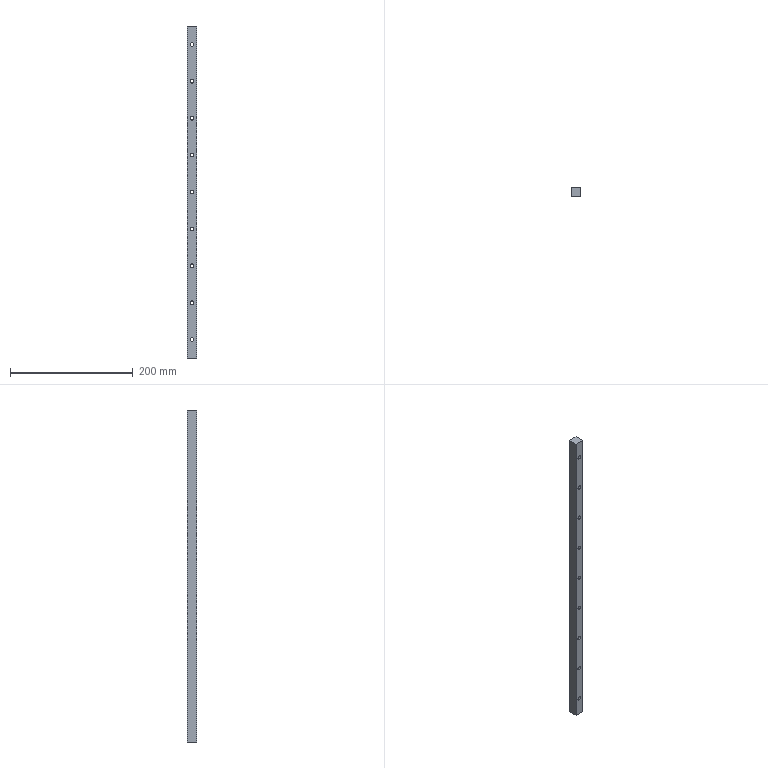Part | 1 solid | 24 faces | box 15 x 15 x 540 mm | volume 117683 mm3 | cylinder 18 | plane 6 | commonest cylinder face diameters 6 x18
STEP:
#1=CARTESIAN_POINT('',(7.5,0.,507.));
#2=VERTEX_POINT('',#1);
#3=CARTESIAN_POINT('',(7.5,0.,513.));
#4=VERTEX_POINT('',#3);
#5=CARTESIAN_POINT('',(7.5,0.,510.));
#6=DIRECTION('',(0.,1.,0.));
#7=DIRECTION('',(0.,0.,1.));
#8=AXIS2_PLACEMENT_3D('',#5,#6,#7);
#9=CIRCLE('',#8,3.);
#10=EDGE_CURVE('',#2,#4,#9,.T.);
#11=ORIENTED_EDGE('',*,*,#10,.F.);
#12=CARTESIAN_POINT('',(7.5,15.,507.));
#13=VERTEX_POINT('',#12);
#14=CARTESIAN_POINT('',(7.5,-35.,507.));
#15=DIRECTION('',(0.,1.,0.));
#16=VECTOR('',#15,1000.);
#17=LINE('',#14,#16);
#18=EDGE_CURVE('',#2,#13,#17,.T.);
#19=ORIENTED_EDGE('',*,*,#18,.T.);
#20=CARTESIAN_POINT('',(7.5,15.,513.));
#21=VERTEX_POINT('',#20);
#22=CARTESIAN_POINT('',(7.5,15.,510.));
#23=DIRECTION('',(0.,1.,0.));
#24=DIRECTION('',(0.,0.,1.));
#25=AXIS2_PLACEMENT_3D('',#22,#23,#24);
#26=CIRCLE('',#25,3.);
#27=EDGE_CURVE('',#13,#21,#26,.T.);
#28=ORIENTED_EDGE('',*,*,#27,.T.);
#29=CARTESIAN_POINT('',(7.5,-35.,513.));
#30=DIRECTION('',(0.,1.,0.));
#31=VECTOR('',#30,1000.);
#32=LINE('',#29,#31);
#33=EDGE_CURVE('',#4,#21,#32,.T.);
#34=ORIENTED_EDGE('',*,*,#33,.F.);
#35=EDGE_LOOP('',(#11,#19,#28,#34));
#36=FACE_OUTER_BOUND('',#35,.T.);
#37=CARTESIAN_POINT('',(7.5,-35.,510.));
#38=DIRECTION('',(0.,1.,0.));
#39=DIRECTION('',(0.,0.,1.));
#40=AXIS2_PLACEMENT_3D('',#37,#38,#39);
#41=CYLINDRICAL_SURFACE('',#40,3.);
#42=ADVANCED_FACE('',(#36),#41,.F.);
#43=CARTESIAN_POINT('',(7.5,0.,447.));
#44=VERTEX_POINT('',#43);
#45=CARTESIAN_POINT('',(7.5,0.,453.));
#46=VERTEX_POINT('',#45);
#47=CARTESIAN_POINT('',(7.5,0.,450.));
#48=DIRECTION('',(0.,1.,0.));
#49=DIRECTION('',(0.,0.,1.));
#50=AXIS2_PLACEMENT_3D('',#47,#48,#49);
#51=CIRCLE('',#50,3.);
#52=EDGE_CURVE('',#44,#46,#51,.T.);
#53=ORIENTED_EDGE('',*,*,#52,.F.);
#54=CARTESIAN_POINT('',(7.5,15.,447.));
#55=VERTEX_POINT('',#54);
#56=CARTESIAN_POINT('',(7.5,-35.,447.));
#57=DIRECTION('',(0.,1.,0.));
#58=VECTOR('',#57,1000.);
#59=LINE('',#56,#58);
#60=EDGE_CURVE('',#44,#55,#59,.T.);
#61=ORIENTED_EDGE('',*,*,#60,.T.);
#62=CARTESIAN_POINT('',(7.5,15.,453.));
#63=VERTEX_POINT('',#62);
#64=CARTESIAN_POINT('',(7.5,15.,450.));
#65=DIRECTION('',(0.,1.,0.));
#66=DIRECTION('',(0.,0.,1.));
#67=AXIS2_PLACEMENT_3D('',#64,#65,#66);
#68=CIRCLE('',#67,3.);
#69=EDGE_CURVE('',#55,#63,#68,.T.);
#70=ORIENTED_EDGE('',*,*,#69,.T.);
#71=CARTESIAN_POINT('',(7.5,-35.,453.));
#72=DIRECTION('',(0.,1.,0.));
#73=VECTOR('',#72,1000.);
#74=LINE('',#71,#73);
#75=EDGE_CURVE('',#46,#63,#74,.T.);
#76=ORIENTED_EDGE('',*,*,#75,.F.);
#77=EDGE_LOOP('',(#53,#61,#70,#76));
#78=FACE_OUTER_BOUND('',#77,.T.);
#79=CARTESIAN_POINT('',(7.5,-35.,450.));
#80=DIRECTION('',(0.,1.,0.));
#81=DIRECTION('',(0.,0.,1.));
#82=AXIS2_PLACEMENT_3D('',#79,#80,#81);
#83=CYLINDRICAL_SURFACE('',#82,3.);
#84=ADVANCED_FACE('',(#78),#83,.F.);
#85=CARTESIAN_POINT('',(7.5,0.,387.));
#86=VERTEX_POINT('',#85);
#87=CARTESIAN_POINT('',(7.5,0.,393.));
#88=VERTEX_POINT('',#87);
#89=CARTESIAN_POINT('',(7.5,0.,390.));
#90=DIRECTION('',(0.,1.,0.));
#91=DIRECTION('',(0.,0.,1.));
#92=AXIS2_PLACEMENT_3D('',#89,#90,#91);
#93=CIRCLE('',#92,3.);
#94=EDGE_CURVE('',#86,#88,#93,.T.);
#95=ORIENTED_EDGE('',*,*,#94,.F.);
#96=CARTESIAN_POINT('',(7.5,15.,387.));
#97=VERTEX_POINT('',#96);
#98=CARTESIAN_POINT('',(7.5,-35.,387.));
#99=DIRECTION('',(0.,1.,0.));
#100=VECTOR('',#99,1000.);
#101=LINE('',#98,#100);
#102=EDGE_CURVE('',#86,#97,#101,.T.);
#103=ORIENTED_EDGE('',*,*,#102,.T.);
#104=CARTESIAN_POINT('',(7.5,15.,393.));
#105=VERTEX_POINT('',#104);
#106=CARTESIAN_POINT('',(7.5,15.,390.));
#107=DIRECTION('',(0.,1.,0.));
#108=DIRECTION('',(0.,0.,1.));
#109=AXIS2_PLACEMENT_3D('',#106,#107,#108);
#110=CIRCLE('',#109,3.);
#111=EDGE_CURVE('',#97,#105,#110,.T.);
#112=ORIENTED_EDGE('',*,*,#111,.T.);
#113=CARTESIAN_POINT('',(7.5,-35.,393.));
#114=DIRECTION('',(0.,1.,0.));
#115=VECTOR('',#114,1000.);
#116=LINE('',#113,#115);
#117=EDGE_CURVE('',#88,#105,#116,.T.);
#118=ORIENTED_EDGE('',*,*,#117,.F.);
#119=EDGE_LOOP('',(#95,#103,#112,#118));
#120=FACE_OUTER_BOUND('',#119,.T.);
#121=CARTESIAN_POINT('',(7.5,-35.,390.));
#122=DIRECTION('',(0.,1.,0.));
#123=DIRECTION('',(0.,0.,1.));
#124=AXIS2_PLACEMENT_3D('',#121,#122,#123);
#125=CYLINDRICAL_SURFACE('',#124,3.);
#126=ADVANCED_FACE('',(#120),#125,.F.);
#127=CARTESIAN_POINT('',(7.5,0.,327.));
#128=VERTEX_POINT('',#127);
#129=CARTESIAN_POINT('',(7.5,0.,333.));
#130=VERTEX_POINT('',#129);
#131=CARTESIAN_POINT('',(7.5,0.,330.));
#132=DIRECTION('',(0.,1.,0.));
#133=DIRECTION('',(0.,0.,1.));
#134=AXIS2_PLACEMENT_3D('',#131,#132,#133);
#135=CIRCLE('',#134,3.);
#136=EDGE_CURVE('',#128,#130,#135,.T.);
#137=ORIENTED_EDGE('',*,*,#136,.F.);
#138=CARTESIAN_POINT('',(7.5,15.,327.));
#139=VERTEX_POINT('',#138);
#140=CARTESIAN_POINT('',(7.5,-35.,327.));
#141=DIRECTION('',(0.,1.,0.));
#142=VECTOR('',#141,1000.);
#143=LINE('',#140,#142);
#144=EDGE_CURVE('',#128,#139,#143,.T.);
#145=ORIENTED_EDGE('',*,*,#144,.T.);
#146=CARTESIAN_POINT('',(7.5,15.,333.));
#147=VERTEX_POINT('',#146);
#148=CARTESIAN_POINT('',(7.5,15.,330.));
#149=DIRECTION('',(0.,1.,0.));
#150=DIRECTION('',(0.,0.,1.));
#151=AXIS2_PLACEMENT_3D('',#148,#149,#150);
#152=CIRCLE('',#151,3.);
#153=EDGE_CURVE('',#139,#147,#152,.T.);
#154=ORIENTED_EDGE('',*,*,#153,.T.);
#155=CARTESIAN_POINT('',(7.5,-35.,333.));
#156=DIRECTION('',(0.,1.,0.));
#157=VECTOR('',#156,1000.);
#158=LINE('',#155,#157);
#159=EDGE_CURVE('',#130,#147,#158,.T.);
#160=ORIENTED_EDGE('',*,*,#159,.F.);
#161=EDGE_LOOP('',(#137,#145,#154,#160));
#162=FACE_OUTER_BOUND('',#161,.T.);
#163=CARTESIAN_POINT('',(7.5,-35.,330.));
#164=DIRECTION('',(0.,1.,0.));
#165=DIRECTION('',(0.,0.,1.));
#166=AXIS2_PLACEMENT_3D('',#163,#164,#165);
#167=CYLINDRICAL_SURFACE('',#166,3.);
#168=ADVANCED_FACE('',(#162),#167,.F.);
#169=CARTESIAN_POINT('',(7.5,0.,267.));
#170=VERTEX_POINT('',#169);
#171=CARTESIAN_POINT('',(7.5,0.,273.));
#172=VERTEX_POINT('',#171);
#173=CARTESIAN_POINT('',(7.5,0.,270.));
#174=DIRECTION('',(0.,1.,0.));
#175=DIRECTION('',(0.,0.,1.));
#176=AXIS2_PLACEMENT_3D('',#173,#174,#175);
#177=CIRCLE('',#176,3.);
#178=EDGE_CURVE('',#170,#172,#177,.T.);
#179=ORIENTED_EDGE('',*,*,#178,.F.);
#180=CARTESIAN_POINT('',(7.5,15.,267.));
#181=VERTEX_POINT('',#180);
#182=CARTESIAN_POINT('',(7.5,-35.,267.));
#183=DIRECTION('',(0.,1.,0.));
#184=VECTOR('',#183,1000.);
#185=LINE('',#182,#184);
#186=EDGE_CURVE('',#170,#181,#185,.T.);
#187=ORIENTED_EDGE('',*,*,#186,.T.);
#188=CARTESIAN_POINT('',(7.5,15.,273.));
#189=VERTEX_POINT('',#188);
#190=CARTESIAN_POINT('',(7.5,15.,270.));
#191=DIRECTION('',(0.,1.,0.));
#192=DIRECTION('',(0.,0.,1.));
#193=AXIS2_PLACEMENT_3D('',#190,#191,#192);
#194=CIRCLE('',#193,3.);
#195=EDGE_CURVE('',#181,#189,#194,.T.);
#196=ORIENTED_EDGE('',*,*,#195,.T.);
#197=CARTESIAN_POINT('',(7.5,-35.,273.));
#198=DIRECTION('',(0.,1.,0.));
#199=VECTOR('',#198,1000.);
#200=LINE('',#197,#199);
#201=EDGE_CURVE('',#172,#189,#200,.T.);
#202=ORIENTED_EDGE('',*,*,#201,.F.);
#203=EDGE_LOOP('',(#179,#187,#196,#202));
#204=FACE_OUTER_BOUND('',#203,.T.);
#205=CARTESIAN_POINT('',(7.5,-35.,270.));
#206=DIRECTION('',(0.,1.,0.));
#207=DIRECTION('',(0.,0.,1.));
#208=AXIS2_PLACEMENT_3D('',#205,#206,#207);
#209=CYLINDRICAL_SURFACE('',#208,3.);
#210=ADVANCED_FACE('',(#204),#209,.F.);
#211=CARTESIAN_POINT('',(7.5,0.,207.));
#212=VERTEX_POINT('',#211);
#213=CARTESIAN_POINT('',(7.5,0.,213.));
#214=VERTEX_POINT('',#213);
#215=CARTESIAN_POINT('',(7.5,0.,210.));
#216=DIRECTION('',(0.,1.,0.));
#217=DIRECTION('',(0.,0.,1.));
#218=AXIS2_PLACEMENT_3D('',#215,#216,#217);
#219=CIRCLE('',#218,3.);
#220=EDGE_CURVE('',#212,#214,#219,.T.);
#221=ORIENTED_EDGE('',*,*,#220,.F.);
#222=CARTESIAN_POINT('',(7.5,15.,207.));
#223=VERTEX_POINT('',#222);
#224=CARTESIAN_POINT('',(7.5,-35.,207.));
#225=DIRECTION('',(0.,1.,0.));
#226=VECTOR('',#225,1000.);
#227=LINE('',#224,#226);
#228=EDGE_CURVE('',#212,#223,#227,.T.);
#229=ORIENTED_EDGE('',*,*,#228,.T.);
#230=CARTESIAN_POINT('',(7.5,15.,213.));
#231=VERTEX_POINT('',#230);
#232=CARTESIAN_POINT('',(7.5,15.,210.));
#233=DIRECTION('',(0.,1.,0.));
#234=DIRECTION('',(0.,0.,1.));
#235=AXIS2_PLACEMENT_3D('',#232,#233,#234);
#236=CIRCLE('',#235,3.);
#237=EDGE_CURVE('',#223,#231,#236,.T.);
#238=ORIENTED_EDGE('',*,*,#237,.T.);
#239=CARTESIAN_POINT('',(7.5,-35.,213.));
#240=DIRECTION('',(0.,1.,0.));
#241=VECTOR('',#240,1000.);
#242=LINE('',#239,#241);
#243=EDGE_CURVE('',#214,#231,#242,.T.);
#244=ORIENTED_EDGE('',*,*,#243,.F.);
#245=EDGE_LOOP('',(#221,#229,#238,#244));
#246=FACE_OUTER_BOUND('',#245,.T.);
#247=CARTESIAN_POINT('',(7.5,-35.,210.));
#248=DIRECTION('',(0.,1.,0.));
#249=DIRECTION('',(0.,0.,1.));
#250=AXIS2_PLACEMENT_3D('',#247,#248,#249);
#251=CYLINDRICAL_SURFACE('',#250,3.);
#252=ADVANCED_FACE('',(#246),#251,.F.);
#253=CARTESIAN_POINT('',(7.5,0.,147.));
#254=VERTEX_POINT('',#253);
#255=CARTESIAN_POINT('',(7.5,0.,153.));
#256=VERTEX_POINT('',#255);
#257=CARTESIAN_POINT('',(7.5,0.,150.));
#258=DIRECTION('',(0.,1.,0.));
#259=DIRECTION('',(0.,0.,1.));
#260=AXIS2_PLACEMENT_3D('',#257,#258,#259);
#261=CIRCLE('',#260,3.);
#262=EDGE_CURVE('',#254,#256,#261,.T.);
#263=ORIENTED_EDGE('',*,*,#262,.F.);
#264=CARTESIAN_POINT('',(7.5,15.,147.));
#265=VERTEX_POINT('',#264);
#266=CARTESIAN_POINT('',(7.5,-35.,147.));
#267=DIRECTION('',(0.,1.,0.));
#268=VECTOR('',#267,1000.);
#269=LINE('',#266,#268);
#270=EDGE_CURVE('',#254,#265,#269,.T.);
#271=ORIENTED_EDGE('',*,*,#270,.T.);
#272=CARTESIAN_POINT('',(7.5,15.,153.));
#273=VERTEX_POINT('',#272);
#274=CARTESIAN_POINT('',(7.5,15.,150.));
#275=DIRECTION('',(0.,1.,0.));
#276=DIRECTION('',(0.,0.,1.));
#277=AXIS2_PLACEMENT_3D('',#274,#275,#276);
#278=CIRCLE('',#277,3.);
#279=EDGE_CURVE('',#265,#273,#278,.T.);
#280=ORIENTED_EDGE('',*,*,#279,.T.);
#281=CARTESIAN_POINT('',(7.5,-35.,153.));
#282=DIRECTION('',(0.,1.,0.));
#283=VECTOR('',#282,1000.);
#284=LINE('',#281,#283);
#285=EDGE_CURVE('',#256,#273,#284,.T.);
#286=ORIENTED_EDGE('',*,*,#285,.F.);
#287=EDGE_LOOP('',(#263,#271,#280,#286));
#288=FACE_OUTER_BOUND('',#287,.T.);
#289=CARTESIAN_POINT('',(7.5,-35.,150.));
#290=DIRECTION('',(0.,1.,0.));
#291=DIRECTION('',(0.,0.,1.));
#292=AXIS2_PLACEMENT_3D('',#289,#290,#291);
#293=CYLINDRICAL_SURFACE('',#292,3.);
#294=ADVANCED_FACE('',(#288),#293,.F.);
#295=CARTESIAN_POINT('',(7.5,0.,87.));
#296=VERTEX_POINT('',#295);
#297=CARTESIAN_POINT('',(7.5,0.,93.));
#298=VERTEX_POINT('',#297);
#299=CARTESIAN_POINT('',(7.5,0.,90.));
#300=DIRECTION('',(0.,1.,0.));
#301=DIRECTION('',(0.,0.,1.));
#302=AXIS2_PLACEMENT_3D('',#299,#300,#301);
#303=CIRCLE('',#302,3.);
#304=EDGE_CURVE('',#296,#298,#303,.T.);
#305=ORIENTED_EDGE('',*,*,#304,.F.);
#306=CARTESIAN_POINT('',(7.5,15.,87.));
#307=VERTEX_POINT('',#306);
#308=CARTESIAN_POINT('',(7.5,-35.,87.));
#309=DIRECTION('',(0.,1.,0.));
#310=VECTOR('',#309,1000.);
#311=LINE('',#308,#310);
#312=EDGE_CURVE('',#296,#307,#311,.T.);
#313=ORIENTED_EDGE('',*,*,#312,.T.);
#314=CARTESIAN_POINT('',(7.5,15.,93.));
#315=VERTEX_POINT('',#314);
#316=CARTESIAN_POINT('',(7.5,15.,90.));
#317=DIRECTION('',(0.,1.,0.));
#318=DIRECTION('',(0.,0.,1.));
#319=AXIS2_PLACEMENT_3D('',#316,#317,#318);
#320=CIRCLE('',#319,3.);
#321=EDGE_CURVE('',#307,#315,#320,.T.);
#322=ORIENTED_EDGE('',*,*,#321,.T.);
#323=CARTESIAN_POINT('',(7.5,-35.,93.));
#324=DIRECTION('',(0.,1.,0.));
#325=VECTOR('',#324,1000.);
#326=LINE('',#323,#325);
#327=EDGE_CURVE('',#298,#315,#326,.T.);
#328=ORIENTED_EDGE('',*,*,#327,.F.);
#329=EDGE_LOOP('',(#305,#313,#322,#328));
#330=FACE_OUTER_BOUND('',#329,.T.);
#331=CARTESIAN_POINT('',(7.5,-35.,90.));
#332=DIRECTION('',(0.,1.,0.));
#333=DIRECTION('',(0.,0.,1.));
#334=AXIS2_PLACEMENT_3D('',#331,#332,#333);
#335=CYLINDRICAL_SURFACE('',#334,3.);
#336=ADVANCED_FACE('',(#330),#335,.F.);
#337=CARTESIAN_POINT('',(7.5,0.,27.));
#338=VERTEX_POINT('',#337);
#339=CARTESIAN_POINT('',(7.5,0.,33.));
#340=VERTEX_POINT('',#339);
#341=CARTESIAN_POINT('',(7.5,0.,30.));
#342=DIRECTION('',(0.,1.,0.));
#343=DIRECTION('',(0.,0.,1.));
#344=AXIS2_PLACEMENT_3D('',#341,#342,#343);
#345=CIRCLE('',#344,3.);
#346=EDGE_CURVE('',#338,#340,#345,.T.);
#347=ORIENTED_EDGE('',*,*,#346,.F.);
#348=CARTESIAN_POINT('',(7.5,15.,27.));
#349=VERTEX_POINT('',#348);
#350=CARTESIAN_POINT('',(7.5,-35.,27.));
#351=DIRECTION('',(0.,1.,0.));
#352=VECTOR('',#351,1000.);
#353=LINE('',#350,#352);
#354=EDGE_CURVE('',#338,#349,#353,.T.);
#355=ORIENTED_EDGE('',*,*,#354,.T.);
#356=CARTESIAN_POINT('',(7.5,15.,33.));
#357=VERTEX_POINT('',#356);
#358=CARTESIAN_POINT('',(7.5,15.,30.));
#359=DIRECTION('',(0.,1.,0.));
#360=DIRECTION('',(0.,0.,1.));
#361=AXIS2_PLACEMENT_3D('',#358,#359,#360);
#362=CIRCLE('',#361,3.);
#363=EDGE_CURVE('',#349,#357,#362,.T.);
#364=ORIENTED_EDGE('',*,*,#363,.T.);
#365=CARTESIAN_POINT('',(7.5,-35.,33.));
#366=DIRECTION('',(0.,1.,0.));
#367=VECTOR('',#366,1000.);
#368=LINE('',#365,#367);
#369=EDGE_CURVE('',#340,#357,#368,.T.);
#370=ORIENTED_EDGE('',*,*,#369,.F.);
#371=EDGE_LOOP('',(#347,#355,#364,#370));
#372=FACE_OUTER_BOUND('',#371,.T.);
#373=CARTESIAN_POINT('',(7.5,-35.,30.));
#374=DIRECTION('',(0.,1.,0.));
#375=DIRECTION('',(0.,0.,1.));
#376=AXIS2_PLACEMENT_3D('',#373,#374,#375);
#377=CYLINDRICAL_SURFACE('',#376,3.);
#378=ADVANCED_FACE('',(#372),#377,.F.);
#379=CARTESIAN_POINT('',(0.,15.,0.));
#380=VERTEX_POINT('',#379);
#381=CARTESIAN_POINT('',(0.,0.,0.));
#382=VERTEX_POINT('',#381);
#383=CARTESIAN_POINT('',(0.,0.,0.));
#384=DIRECTION('',(0.,-1.,0.));
#385=VECTOR('',#384,1000.);
#386=LINE('',#383,#385);
#387=EDGE_CURVE('',#380,#382,#386,.T.);
#388=ORIENTED_EDGE('',*,*,#387,.T.);
#389=CARTESIAN_POINT('',(0.,0.,540.));
#390=VERTEX_POINT('',#389);
#391=CARTESIAN_POINT('',(0.,0.,540.));
#392=DIRECTION('',(0.,0.,-1.));
#393=VECTOR('',#392,1000.);
#394=LINE('',#391,#393);
#395=EDGE_CURVE('',#390,#382,#394,.T.);
#396=ORIENTED_EDGE('',*,*,#395,.F.);
#397=CARTESIAN_POINT('',(0.,15.,540.));
#398=VERTEX_POINT('',#397);
#399=CARTESIAN_POINT('',(0.,0.,540.));
#400=DIRECTION('',(0.,-1.,0.));
#401=VECTOR('',#400,1000.);
#402=LINE('',#399,#401);
#403=EDGE_CURVE('',#398,#390,#402,.T.);
#404=ORIENTED_EDGE('',*,*,#403,.F.);
#405=CARTESIAN_POINT('',(0.,15.,540.));
#406=DIRECTION('',(0.,0.,-1.));
#407=VECTOR('',#406,1000.);
#408=LINE('',#405,#407);
#409=EDGE_CURVE('',#398,#380,#408,.T.);
#410=ORIENTED_EDGE('',*,*,#409,.T.);
#411=EDGE_LOOP('',(#388,#396,#404,#410));
#412=FACE_OUTER_BOUND('',#411,.T.);
#413=CARTESIAN_POINT('',(0.,0.,540.));
#414=DIRECTION('',(1.,0.,0.));
#415=DIRECTION('',(0.,0.,-1.));
#416=AXIS2_PLACEMENT_3D('',#413,#414,#415);
#417=PLANE('',#416);
#418=ADVANCED_FACE('',(#412),#417,.F.);
#419=CARTESIAN_POINT('',(7.5,0.,90.));
#420=DIRECTION('',(0.,1.,0.));
#421=DIRECTION('',(0.,0.,1.));
#422=AXIS2_PLACEMENT_3D('',#419,#420,#421);
#423=CIRCLE('',#422,3.);
#424=EDGE_CURVE('',#298,#296,#423,.T.);
#425=ORIENTED_EDGE('',*,*,#424,.T.);
#426=ORIENTED_EDGE('',*,*,#304,.T.);
#427=EDGE_LOOP('',(#425,#426));
#428=FACE_BOUND('',#427,.T.);
#429=CARTESIAN_POINT('',(7.5,0.,30.));
#430=DIRECTION('',(0.,1.,0.));
#431=DIRECTION('',(0.,0.,1.));
#432=AXIS2_PLACEMENT_3D('',#429,#430,#431);
#433=CIRCLE('',#432,3.);
#434=EDGE_CURVE('',#340,#338,#433,.T.);
#435=ORIENTED_EDGE('',*,*,#434,.T.);
#436=ORIENTED_EDGE('',*,*,#346,.T.);
#437=EDGE_LOOP('',(#435,#436));
#438=FACE_BOUND('',#437,.T.);
#439=CARTESIAN_POINT('',(15.,0.,0.));
#440=VERTEX_POINT('',#439);
#441=CARTESIAN_POINT('',(0.,0.,0.));
#442=DIRECTION('',(1.,0.,0.));
#443=VECTOR('',#442,1000.);
#444=LINE('',#441,#443);
#445=EDGE_CURVE('',#382,#440,#444,.T.);
#446=ORIENTED_EDGE('',*,*,#445,.T.);
#447=CARTESIAN_POINT('',(15.,0.,540.));
#448=VERTEX_POINT('',#447);
#449=CARTESIAN_POINT('',(15.,0.,540.));
#450=DIRECTION('',(0.,0.,-1.));
#451=VECTOR('',#450,1000.);
#452=LINE('',#449,#451);
#453=EDGE_CURVE('',#448,#440,#452,.T.);
#454=ORIENTED_EDGE('',*,*,#453,.F.);
#455=CARTESIAN_POINT('',(0.,0.,540.));
#456=DIRECTION('',(1.,0.,0.));
#457=VECTOR('',#456,1000.);
#458=LINE('',#455,#457);
#459=EDGE_CURVE('',#390,#448,#458,.T.);
#460=ORIENTED_EDGE('',*,*,#459,.F.);
#461=ORIENTED_EDGE('',*,*,#395,.T.);
#462=EDGE_LOOP('',(#446,#454,#460,#461));
#463=FACE_OUTER_BOUND('',#462,.T.);
#464=CARTESIAN_POINT('',(7.5,0.,150.));
#465=DIRECTION('',(0.,1.,0.));
#466=DIRECTION('',(0.,0.,1.));
#467=AXIS2_PLACEMENT_3D('',#464,#465,#466);
#468=CIRCLE('',#467,3.);
#469=EDGE_CURVE('',#256,#254,#468,.T.);
#470=ORIENTED_EDGE('',*,*,#469,.T.);
#471=ORIENTED_EDGE('',*,*,#262,.T.);
#472=EDGE_LOOP('',(#470,#471));
#473=FACE_BOUND('',#472,.T.);
#474=CARTESIAN_POINT('',(7.5,0.,210.));
#475=DIRECTION('',(0.,1.,0.));
#476=DIRECTION('',(0.,0.,1.));
#477=AXIS2_PLACEMENT_3D('',#474,#475,#476);
#478=CIRCLE('',#477,3.);
#479=EDGE_CURVE('',#214,#212,#478,.T.);
#480=ORIENTED_EDGE('',*,*,#479,.T.);
#481=ORIENTED_EDGE('',*,*,#220,.T.);
#482=EDGE_LOOP('',(#480,#481));
#483=FACE_BOUND('',#482,.T.);
#484=CARTESIAN_POINT('',(7.5,0.,270.));
#485=DIRECTION('',(0.,1.,0.));
#486=DIRECTION('',(0.,0.,1.));
#487=AXIS2_PLACEMENT_3D('',#484,#485,#486);
#488=CIRCLE('',#487,3.);
#489=EDGE_CURVE('',#172,#170,#488,.T.);
#490=ORIENTED_EDGE('',*,*,#489,.T.);
#491=ORIENTED_EDGE('',*,*,#178,.T.);
#492=EDGE_LOOP('',(#490,#491));
#493=FACE_BOUND('',#492,.T.);
#494=CARTESIAN_POINT('',(7.5,0.,330.));
#495=DIRECTION('',(0.,1.,0.));
#496=DIRECTION('',(0.,0.,1.));
#497=AXIS2_PLACEMENT_3D('',#494,#495,#496);
#498=CIRCLE('',#497,3.);
#499=EDGE_CURVE('',#130,#128,#498,.T.);
#500=ORIENTED_EDGE('',*,*,#499,.T.);
#501=ORIENTED_EDGE('',*,*,#136,.T.);
#502=EDGE_LOOP('',(#500,#501));
#503=FACE_BOUND('',#502,.T.);
#504=CARTESIAN_POINT('',(7.5,0.,390.));
#505=DIRECTION('',(0.,1.,0.));
#506=DIRECTION('',(0.,0.,1.));
#507=AXIS2_PLACEMENT_3D('',#504,#505,#506);
#508=CIRCLE('',#507,3.);
#509=EDGE_CURVE('',#88,#86,#508,.T.);
#510=ORIENTED_EDGE('',*,*,#509,.T.);
#511=ORIENTED_EDGE('',*,*,#94,.T.);
#512=EDGE_LOOP('',(#510,#511));
#513=FACE_BOUND('',#512,.T.);
#514=CARTESIAN_POINT('',(7.5,0.,450.));
#515=DIRECTION('',(0.,1.,0.));
#516=DIRECTION('',(0.,0.,1.));
#517=AXIS2_PLACEMENT_3D('',#514,#515,#516);
#518=CIRCLE('',#517,3.);
#519=EDGE_CURVE('',#46,#44,#518,.T.);
#520=ORIENTED_EDGE('',*,*,#519,.T.);
#521=ORIENTED_EDGE('',*,*,#52,.T.);
#522=EDGE_LOOP('',(#520,#521));
#523=FACE_BOUND('',#522,.T.);
#524=CARTESIAN_POINT('',(7.5,0.,510.));
#525=DIRECTION('',(0.,1.,0.));
#526=DIRECTION('',(0.,0.,1.));
#527=AXIS2_PLACEMENT_3D('',#524,#525,#526);
#528=CIRCLE('',#527,3.);
#529=EDGE_CURVE('',#4,#2,#528,.T.);
#530=ORIENTED_EDGE('',*,*,#529,.T.);
#531=ORIENTED_EDGE('',*,*,#10,.T.);
#532=EDGE_LOOP('',(#530,#531));
#533=FACE_BOUND('',#532,.T.);
#534=CARTESIAN_POINT('',(0.,0.,540.));
#535=DIRECTION('',(0.,1.,0.));
#536=DIRECTION('',(0.,0.,1.));
#537=AXIS2_PLACEMENT_3D('',#534,#535,#536);
#538=PLANE('',#537);
#539=ADVANCED_FACE('',(#428,#438,#463,#473,#483,#493,#503,#513,#523,#533),#538,.F.);
#540=CARTESIAN_POINT('',(15.,15.,0.));
#541=VERTEX_POINT('',#540);
#542=CARTESIAN_POINT('',(15.,0.,0.));
#543=DIRECTION('',(0.,1.,0.));
#544=VECTOR('',#543,1000.);
#545=LINE('',#542,#544);
#546=EDGE_CURVE('',#440,#541,#545,.T.);
#547=ORIENTED_EDGE('',*,*,#546,.T.);
#548=CARTESIAN_POINT('',(15.,15.,540.));
#549=VERTEX_POINT('',#548);
#550=CARTESIAN_POINT('',(15.,15.,540.));
#551=DIRECTION('',(0.,0.,-1.));
#552=VECTOR('',#551,1000.);
#553=LINE('',#550,#552);
#554=EDGE_CURVE('',#549,#541,#553,.T.);
#555=ORIENTED_EDGE('',*,*,#554,.F.);
#556=CARTESIAN_POINT('',(15.,0.,540.));
#557=DIRECTION('',(0.,1.,0.));
#558=VECTOR('',#557,1000.);
#559=LINE('',#556,#558);
#560=EDGE_CURVE('',#448,#549,#559,.T.);
#561=ORIENTED_EDGE('',*,*,#560,.F.);
#562=ORIENTED_EDGE('',*,*,#453,.T.);
#563=EDGE_LOOP('',(#547,#555,#561,#562));
#564=FACE_OUTER_BOUND('',#563,.T.);
#565=CARTESIAN_POINT('',(15.,0.,540.));
#566=DIRECTION('',(-1.,0.,0.));
#567=DIRECTION('',(0.,0.,1.));
#568=AXIS2_PLACEMENT_3D('',#565,#566,#567);
#569=PLANE('',#568);
#570=ADVANCED_FACE('',(#564),#569,.F.);
#571=CARTESIAN_POINT('',(7.5,15.,90.));
#572=DIRECTION('',(0.,1.,0.));
#573=DIRECTION('',(0.,0.,1.));
#574=AXIS2_PLACEMENT_3D('',#571,#572,#573);
#575=CIRCLE('',#574,3.);
#576=EDGE_CURVE('',#315,#307,#575,.T.);
#577=ORIENTED_EDGE('',*,*,#576,.F.);
#578=ORIENTED_EDGE('',*,*,#321,.F.);
#579=EDGE_LOOP('',(#577,#578));
#580=FACE_BOUND('',#579,.T.);
#581=CARTESIAN_POINT('',(7.5,15.,30.));
#582=DIRECTION('',(0.,1.,0.));
#583=DIRECTION('',(0.,0.,1.));
#584=AXIS2_PLACEMENT_3D('',#581,#582,#583);
#585=CIRCLE('',#584,3.);
#586=EDGE_CURVE('',#357,#349,#585,.T.);
#587=ORIENTED_EDGE('',*,*,#586,.F.);
#588=ORIENTED_EDGE('',*,*,#363,.F.);
#589=EDGE_LOOP('',(#587,#588));
#590=FACE_BOUND('',#589,.T.);
#591=CARTESIAN_POINT('',(0.,15.,0.));
#592=DIRECTION('',(-1.,0.,0.));
#593=VECTOR('',#592,1000.);
#594=LINE('',#591,#593);
#595=EDGE_CURVE('',#541,#380,#594,.T.);
#596=ORIENTED_EDGE('',*,*,#595,.T.);
#597=ORIENTED_EDGE('',*,*,#409,.F.);
#598=CARTESIAN_POINT('',(0.,15.,540.));
#599=DIRECTION('',(-1.,0.,0.));
#600=VECTOR('',#599,1000.);
#601=LINE('',#598,#600);
#602=EDGE_CURVE('',#549,#398,#601,.T.);
#603=ORIENTED_EDGE('',*,*,#602,.F.);
#604=ORIENTED_EDGE('',*,*,#554,.T.);
#605=EDGE_LOOP('',(#596,#597,#603,#604));
#606=FACE_OUTER_BOUND('',#605,.T.);
#607=CARTESIAN_POINT('',(7.5,15.,150.));
#608=DIRECTION('',(0.,1.,0.));
#609=DIRECTION('',(0.,0.,1.));
#610=AXIS2_PLACEMENT_3D('',#607,#608,#609);
#611=CIRCLE('',#610,3.);
#612=EDGE_CURVE('',#273,#265,#611,.T.);
#613=ORIENTED_EDGE('',*,*,#612,.F.);
#614=ORIENTED_EDGE('',*,*,#279,.F.);
#615=EDGE_LOOP('',(#613,#614));
#616=FACE_BOUND('',#615,.T.);
#617=CARTESIAN_POINT('',(7.5,15.,210.));
#618=DIRECTION('',(0.,1.,0.));
#619=DIRECTION('',(0.,0.,1.));
#620=AXIS2_PLACEMENT_3D('',#617,#618,#619);
#621=CIRCLE('',#620,3.);
#622=EDGE_CURVE('',#231,#223,#621,.T.);
#623=ORIENTED_EDGE('',*,*,#622,.F.);
#624=ORIENTED_EDGE('',*,*,#237,.F.);
#625=EDGE_LOOP('',(#623,#624));
#626=FACE_BOUND('',#625,.T.);
#627=CARTESIAN_POINT('',(7.5,15.,270.));
#628=DIRECTION('',(0.,1.,0.));
#629=DIRECTION('',(0.,0.,1.));
#630=AXIS2_PLACEMENT_3D('',#627,#628,#629);
#631=CIRCLE('',#630,3.);
#632=EDGE_CURVE('',#189,#181,#631,.T.);
#633=ORIENTED_EDGE('',*,*,#632,.F.);
#634=ORIENTED_EDGE('',*,*,#195,.F.);
#635=EDGE_LOOP('',(#633,#634));
#636=FACE_BOUND('',#635,.T.);
#637=CARTESIAN_POINT('',(7.5,15.,330.));
#638=DIRECTION('',(0.,1.,0.));
#639=DIRECTION('',(0.,0.,1.));
#640=AXIS2_PLACEMENT_3D('',#637,#638,#639);
#641=CIRCLE('',#640,3.);
#642=EDGE_CURVE('',#147,#139,#641,.T.);
#643=ORIENTED_EDGE('',*,*,#642,.F.);
#644=ORIENTED_EDGE('',*,*,#153,.F.);
#645=EDGE_LOOP('',(#643,#644));
#646=FACE_BOUND('',#645,.T.);
#647=CARTESIAN_POINT('',(7.5,15.,390.));
#648=DIRECTION('',(0.,1.,0.));
#649=DIRECTION('',(0.,0.,1.));
#650=AXIS2_PLACEMENT_3D('',#647,#648,#649);
#651=CIRCLE('',#650,3.);
#652=EDGE_CURVE('',#105,#97,#651,.T.);
#653=ORIENTED_EDGE('',*,*,#652,.F.);
#654=ORIENTED_EDGE('',*,*,#111,.F.);
#655=EDGE_LOOP('',(#653,#654));
#656=FACE_BOUND('',#655,.T.);
#657=CARTESIAN_POINT('',(7.5,15.,450.));
#658=DIRECTION('',(0.,1.,0.));
#659=DIRECTION('',(0.,0.,1.));
#660=AXIS2_PLACEMENT_3D('',#657,#658,#659);
#661=CIRCLE('',#660,3.);
#662=EDGE_CURVE('',#63,#55,#661,.T.);
#663=ORIENTED_EDGE('',*,*,#662,.F.);
#664=ORIENTED_EDGE('',*,*,#69,.F.);
#665=EDGE_LOOP('',(#663,#664));
#666=FACE_BOUND('',#665,.T.);
#667=CARTESIAN_POINT('',(7.5,15.,510.));
#668=DIRECTION('',(0.,1.,0.));
#669=DIRECTION('',(0.,0.,1.));
#670=AXIS2_PLACEMENT_3D('',#667,#668,#669);
#671=CIRCLE('',#670,3.);
#672=EDGE_CURVE('',#21,#13,#671,.T.);
#673=ORIENTED_EDGE('',*,*,#672,.F.);
#674=ORIENTED_EDGE('',*,*,#27,.F.);
#675=EDGE_LOOP('',(#673,#674));
#676=FACE_BOUND('',#675,.T.);
#677=CARTESIAN_POINT('',(0.,15.,540.));
#678=DIRECTION('',(0.,-1.,0.));
#679=DIRECTION('',(0.,0.,-1.));
#680=AXIS2_PLACEMENT_3D('',#677,#678,#679);
#681=PLANE('',#680);
#682=ADVANCED_FACE('',(#580,#590,#606,#616,#626,#636,#646,#656,#666,#676),#681,.F.);
#683=ORIENTED_EDGE('',*,*,#403,.T.);
#684=ORIENTED_EDGE('',*,*,#459,.T.);
#685=ORIENTED_EDGE('',*,*,#560,.T.);
#686=ORIENTED_EDGE('',*,*,#602,.T.);
#687=EDGE_LOOP('',(#683,#684,#685,#686));
#688=FACE_OUTER_BOUND('',#687,.T.);
#689=CARTESIAN_POINT('',(0.,0.,540.));
#690=DIRECTION('',(0.,0.,-1.));
#691=DIRECTION('',(-1.,0.,0.));
#692=AXIS2_PLACEMENT_3D('',#689,#690,#691);
#693=PLANE('',#692);
#694=ADVANCED_FACE('',(#688),#693,.F.);
#695=ORIENTED_EDGE('',*,*,#387,.F.);
#696=ORIENTED_EDGE('',*,*,#595,.F.);
#697=ORIENTED_EDGE('',*,*,#546,.F.);
#698=ORIENTED_EDGE('',*,*,#445,.F.);
#699=EDGE_LOOP('',(#695,#696,#697,#698));
#700=FACE_OUTER_BOUND('',#699,.T.);
#701=CARTESIAN_POINT('',(0.,0.,0.));
#702=DIRECTION('',(0.,0.,-1.));
#703=DIRECTION('',(-1.,0.,0.));
#704=AXIS2_PLACEMENT_3D('',#701,#702,#703);
#705=PLANE('',#704);
#706=ADVANCED_FACE('',(#700),#705,.T.);
#707=ORIENTED_EDGE('',*,*,#354,.F.);
#708=ORIENTED_EDGE('',*,*,#434,.F.);
#709=ORIENTED_EDGE('',*,*,#369,.T.);
#710=ORIENTED_EDGE('',*,*,#586,.T.);
#711=EDGE_LOOP('',(#707,#708,#709,#710));
#712=FACE_OUTER_BOUND('',#711,.T.);
#713=CARTESIAN_POINT('',(7.5,-35.,30.));
#714=DIRECTION('',(0.,1.,0.));
#715=DIRECTION('',(0.,0.,1.));
#716=AXIS2_PLACEMENT_3D('',#713,#714,#715);
#717=CYLINDRICAL_SURFACE('',#716,3.);
#718=ADVANCED_FACE('',(#712),#717,.F.);
#719=ORIENTED_EDGE('',*,*,#312,.F.);
#720=ORIENTED_EDGE('',*,*,#424,.F.);
#721=ORIENTED_EDGE('',*,*,#327,.T.);
#722=ORIENTED_EDGE('',*,*,#576,.T.);
#723=EDGE_LOOP('',(#719,#720,#721,#722));
#724=FACE_OUTER_BOUND('',#723,.T.);
#725=CARTESIAN_POINT('',(7.5,-35.,90.));
#726=DIRECTION('',(0.,1.,0.));
#727=DIRECTION('',(0.,0.,1.));
#728=AXIS2_PLACEMENT_3D('',#725,#726,#727);
#729=CYLINDRICAL_SURFACE('',#728,3.);
#730=ADVANCED_FACE('',(#724),#729,.F.);
#731=ORIENTED_EDGE('',*,*,#270,.F.);
#732=ORIENTED_EDGE('',*,*,#469,.F.);
#733=ORIENTED_EDGE('',*,*,#285,.T.);
#734=ORIENTED_EDGE('',*,*,#612,.T.);
#735=EDGE_LOOP('',(#731,#732,#733,#734));
#736=FACE_OUTER_BOUND('',#735,.T.);
#737=CARTESIAN_POINT('',(7.5,-35.,150.));
#738=DIRECTION('',(0.,1.,0.));
#739=DIRECTION('',(0.,0.,1.));
#740=AXIS2_PLACEMENT_3D('',#737,#738,#739);
#741=CYLINDRICAL_SURFACE('',#740,3.);
#742=ADVANCED_FACE('',(#736),#741,.F.);
#743=ORIENTED_EDGE('',*,*,#228,.F.);
#744=ORIENTED_EDGE('',*,*,#479,.F.);
#745=ORIENTED_EDGE('',*,*,#243,.T.);
#746=ORIENTED_EDGE('',*,*,#622,.T.);
#747=EDGE_LOOP('',(#743,#744,#745,#746));
#748=FACE_OUTER_BOUND('',#747,.T.);
#749=CARTESIAN_POINT('',(7.5,-35.,210.));
#750=DIRECTION('',(0.,1.,0.));
#751=DIRECTION('',(0.,0.,1.));
#752=AXIS2_PLACEMENT_3D('',#749,#750,#751);
#753=CYLINDRICAL_SURFACE('',#752,3.);
#754=ADVANCED_FACE('',(#748),#753,.F.);
#755=ORIENTED_EDGE('',*,*,#186,.F.);
#756=ORIENTED_EDGE('',*,*,#489,.F.);
#757=ORIENTED_EDGE('',*,*,#201,.T.);
#758=ORIENTED_EDGE('',*,*,#632,.T.);
#759=EDGE_LOOP('',(#755,#756,#757,#758));
#760=FACE_OUTER_BOUND('',#759,.T.);
#761=CARTESIAN_POINT('',(7.5,-35.,270.));
#762=DIRECTION('',(0.,1.,0.));
#763=DIRECTION('',(0.,0.,1.));
#764=AXIS2_PLACEMENT_3D('',#761,#762,#763);
#765=CYLINDRICAL_SURFACE('',#764,3.);
#766=ADVANCED_FACE('',(#760),#765,.F.);
#767=ORIENTED_EDGE('',*,*,#144,.F.);
#768=ORIENTED_EDGE('',*,*,#499,.F.);
#769=ORIENTED_EDGE('',*,*,#159,.T.);
#770=ORIENTED_EDGE('',*,*,#642,.T.);
#771=EDGE_LOOP('',(#767,#768,#769,#770));
#772=FACE_OUTER_BOUND('',#771,.T.);
#773=CARTESIAN_POINT('',(7.5,-35.,330.));
#774=DIRECTION('',(0.,1.,0.));
#775=DIRECTION('',(0.,0.,1.));
#776=AXIS2_PLACEMENT_3D('',#773,#774,#775);
#777=CYLINDRICAL_SURFACE('',#776,3.);
#778=ADVANCED_FACE('',(#772),#777,.F.);
#779=ORIENTED_EDGE('',*,*,#102,.F.);
#780=ORIENTED_EDGE('',*,*,#509,.F.);
#781=ORIENTED_EDGE('',*,*,#117,.T.);
#782=ORIENTED_EDGE('',*,*,#652,.T.);
#783=EDGE_LOOP('',(#779,#780,#781,#782));
#784=FACE_OUTER_BOUND('',#783,.T.);
#785=CARTESIAN_POINT('',(7.5,-35.,390.));
#786=DIRECTION('',(0.,1.,0.));
#787=DIRECTION('',(0.,0.,1.));
#788=AXIS2_PLACEMENT_3D('',#785,#786,#787);
#789=CYLINDRICAL_SURFACE('',#788,3.);
#790=ADVANCED_FACE('',(#784),#789,.F.);
#791=ORIENTED_EDGE('',*,*,#60,.F.);
#792=ORIENTED_EDGE('',*,*,#519,.F.);
#793=ORIENTED_EDGE('',*,*,#75,.T.);
#794=ORIENTED_EDGE('',*,*,#662,.T.);
#795=EDGE_LOOP('',(#791,#792,#793,#794));
#796=FACE_OUTER_BOUND('',#795,.T.);
#797=CARTESIAN_POINT('',(7.5,-35.,450.));
#798=DIRECTION('',(0.,1.,0.));
#799=DIRECTION('',(0.,0.,1.));
#800=AXIS2_PLACEMENT_3D('',#797,#798,#799);
#801=CYLINDRICAL_SURFACE('',#800,3.);
#802=ADVANCED_FACE('',(#796),#801,.F.);
#803=ORIENTED_EDGE('',*,*,#18,.F.);
#804=ORIENTED_EDGE('',*,*,#529,.F.);
#805=ORIENTED_EDGE('',*,*,#33,.T.);
#806=ORIENTED_EDGE('',*,*,#672,.T.);
#807=EDGE_LOOP('',(#803,#804,#805,#806));
#808=FACE_OUTER_BOUND('',#807,.T.);
#809=CARTESIAN_POINT('',(7.5,-35.,510.));
#810=DIRECTION('',(0.,1.,0.));
#811=DIRECTION('',(0.,0.,1.));
#812=AXIS2_PLACEMENT_3D('',#809,#810,#811);
#813=CYLINDRICAL_SURFACE('',#812,3.);
#814=ADVANCED_FACE('',(#808),#813,.F.);
#815=CLOSED_SHELL('',(#42,#84,#126,#168,#210,#252,#294,#336,#378,#418,#539,#570,#682,#694,#706,#718,#730,#742,#754,#766,#778,#790,#802,#814));
#816=MANIFOLD_SOLID_BREP('',#815);
#817=CARTESIAN_POINT('',(0.,0.,0.));
#818=DIRECTION('',(0.,0.,1.));
#819=DIRECTION('',(1.,0.,0.));
#820=AXIS2_PLACEMENT_3D('',#817,#818,#819);
#821=(LENGTH_UNIT()NAMED_UNIT(*)SI_UNIT(.MILLI.,.METRE.));
#822=UNCERTAINTY_MEASURE_WITH_UNIT(LENGTH_MEASURE(0.00001),#821,'','');
#823=(NAMED_UNIT(*)PLANE_ANGLE_UNIT()SI_UNIT($,.RADIAN.));
#824=(NAMED_UNIT(*)SI_UNIT($,.STERADIAN.)SOLID_ANGLE_UNIT());
#825=(GEOMETRIC_REPRESENTATION_CONTEXT(3)GLOBAL_UNCERTAINTY_ASSIGNED_CONTEXT((#822))GLOBAL_UNIT_ASSIGNED_CONTEXT((#821,#823,#824))REPRESENTATION_CONTEXT('',''));
#826=ADVANCED_BREP_SHAPE_REPRESENTATION('',(#816,#820),#825);